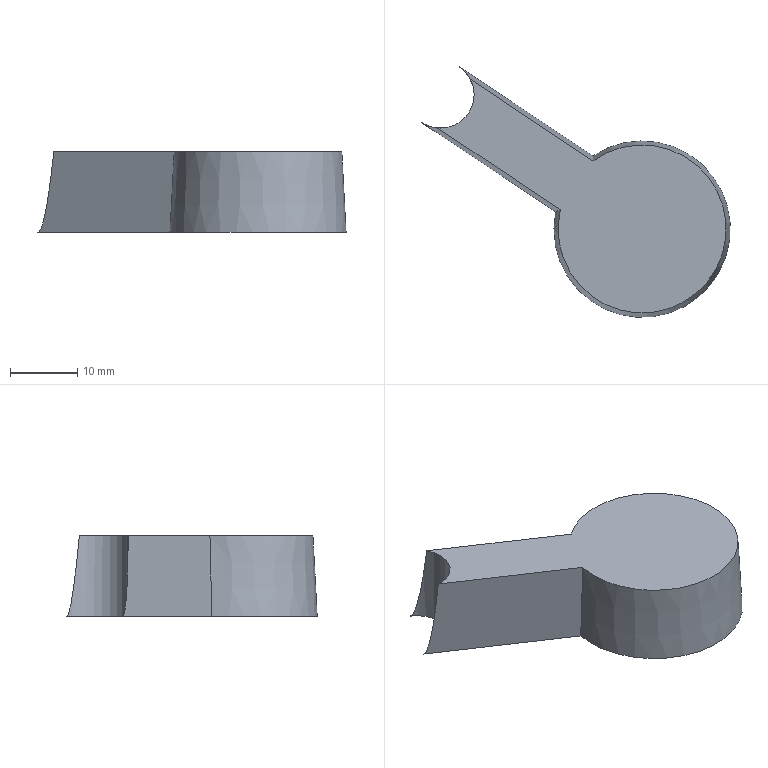Part | STEP file | solid 114 | 1 solid | 6 faces | box 45.902 x 37.289 x 12 mm | volume 8376 mm3 | plane 4 | cone 1 | cylinder 1 | commonest cylinder face diameters 10 x1